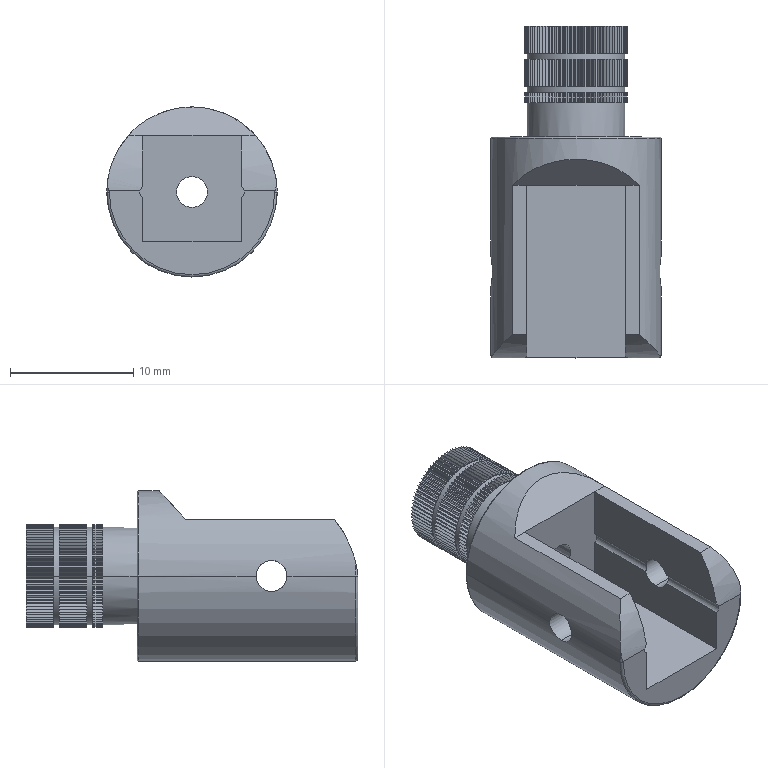Part | SolidWorks | features ICE 7, Fillet 2, CirPattern 1, RevCut 1, Revolution 1 | 1 solid | 916 faces | box 13.8 x 26.9 x 13.8 mm | volume 1584 mm3 | plane 893 | cylinder 18 | torus 5 | commonest cylinder face diameters 2.5 x6 1 x4 6.5 x2 7.9 x2 13.8 x2 18 x2